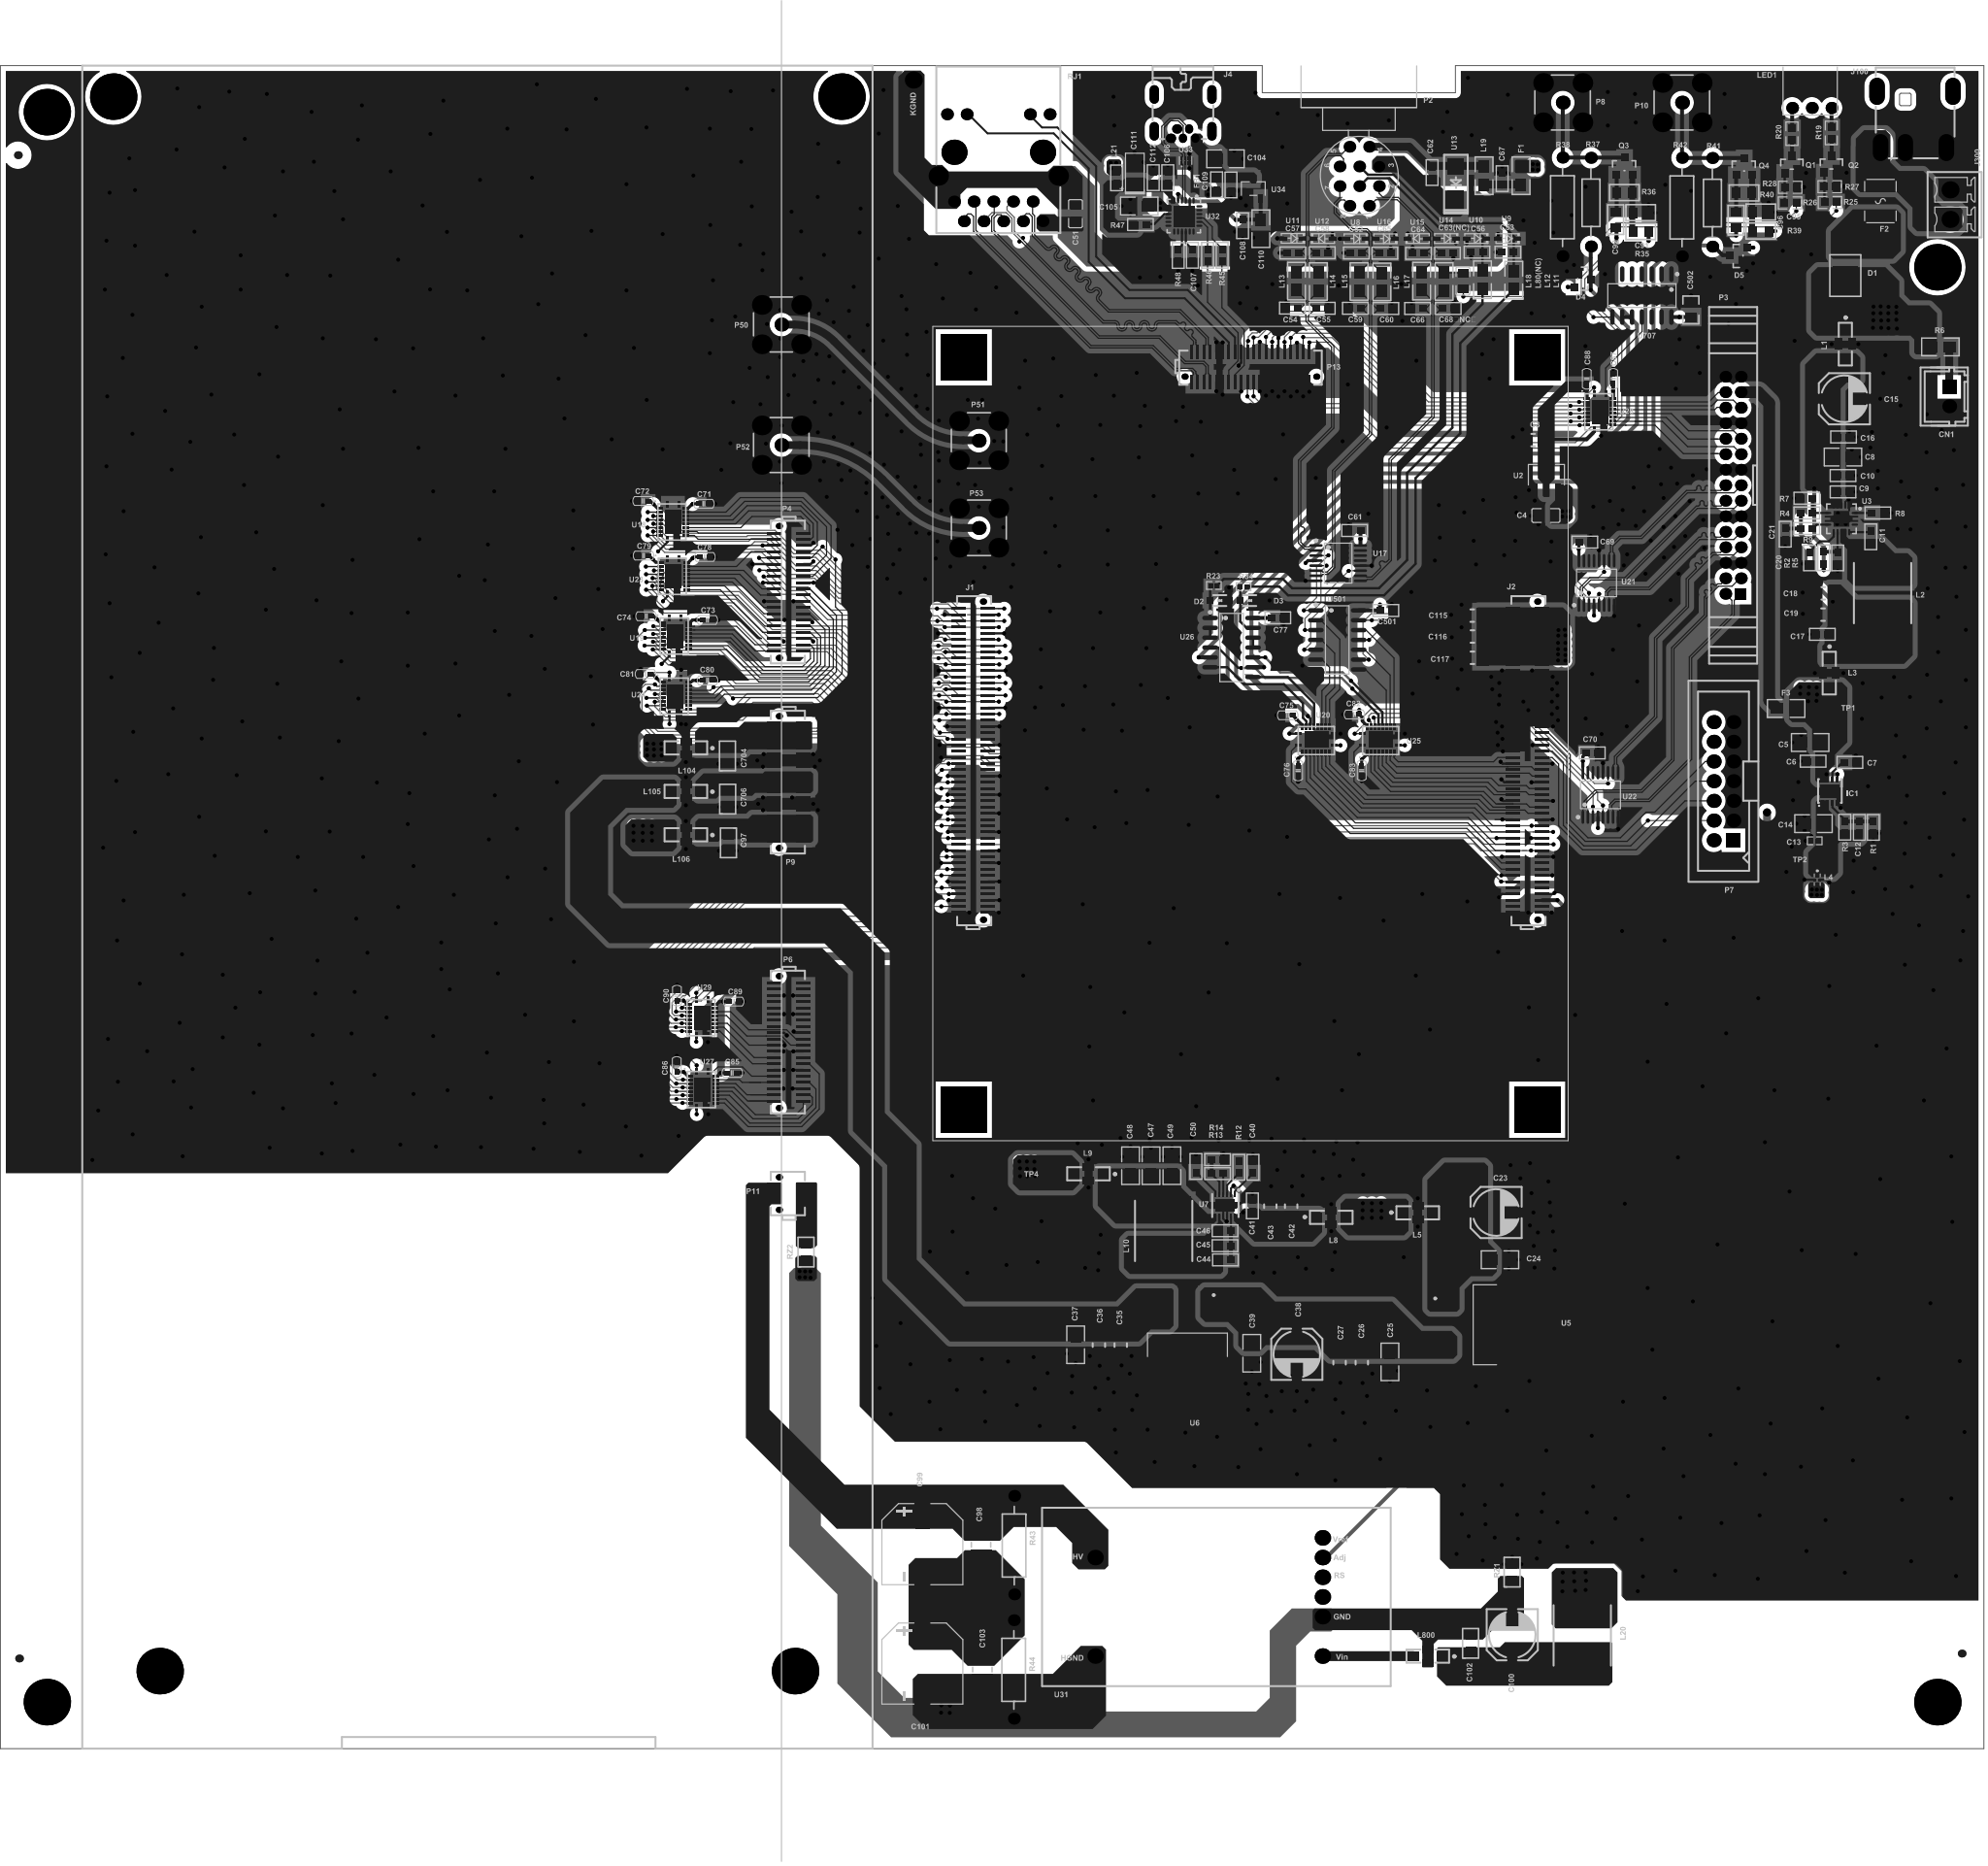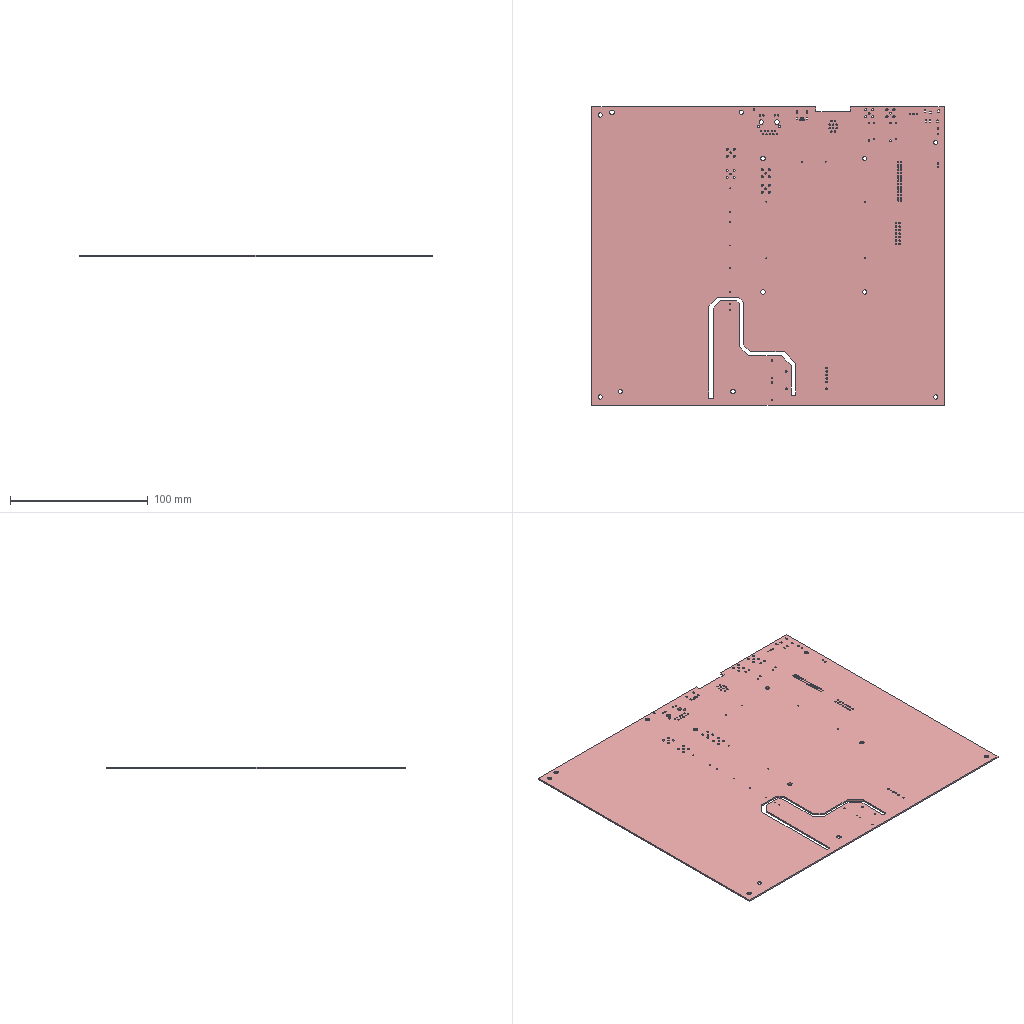Circuit board layout | Altium Designer | box 256 x 217 x 1.1 mm
Layer stack:
# Altium Designer layer stack of  (unit mm; dielectric type: 0 none, 1 core, 2 prepreg, 3 surface material)
index,name,kind,layer,copper_thickness_mm,dielectric_type,dielectric_thickness_mm,dielectric_material,dielectric_constant
0,Top Paste,other,,,,,,
1,Top Overlay,other,,,,,,
2,Top Solder,dielectric,,,3,0.0102,Solder Resist,3.5
3,Top Layer,copper,Top Layer,0.0356,,,,
4,Dielectric1,dielectric,,,1,0.32,FR-4,4.8
5,GND,copper,GND,0.0356,,,,
6,Dielectric5,dielectric,,,2,0.32,FR-4,4.8
7,POWER,copper,POWER,0.0356,,,,
8,Dielectric6,dielectric,,,1,0.32,FR-4,4.8
9,Bottom Layer,copper,Bottom Layer,0.0356,,,,
10,Bottom Solder,dielectric,,,3,0.0102,Solder Resist,3.5
11,Bottom Overlay,other,,,,,,
12,Bottom Paste,other,,,,,,
# drill layer pairs: low layer,high layer
drill_pair,Top Layer,Bottom Layer
Part placement:
Designator,Comment,Layer,Footprint,Center-X(mm),Center-Y(mm),Rotation
U3,#NAME?,TopLayer,VQFN-14_L3.5-W3.5-P0.50-BL-EP_TPS54622RHLT,231.619,152.568,180
R6,0R1%,TopLayer,0805,244.387,174.729,360
CN1,#NAME?,TopLayer,CONN-TH_2P-P2.50_HX25003-2A,245.53,168.328,270
C103,1KV/1nF,TopLayer,3225[1210],120.739,4.193,270
C98,1KV/1nF,TopLayer,3225[1210],120.568,20.289,270
F2,16V 4A,TopLayer,1812,236.646,193.534,270
C3,22uf,TopLayer,1206,191.841,162.818,270
C4,10uf,TopLayer,0805A,193.517,152.937,90
C5,22uF/16V,TopLayer,0805,227.578,123.727,360
C6,100nF,TopLayer,0603,227.959,121.314,90
C7,100nF,TopLayer,0603,232.709,121.162,270
C8,10uF 25V,TopLayer,0805,231.814,160.53,360
C9,4.7uF 25V,TopLayer,0603,231.82,156.036,90
C10,100nF 25V,TopLayer,0603,231.82,158.144,90
C11,100nF 25V,TopLayer,0603,235.402,150.245,360
C12,10nF,TopLayer,0603,233.928,112.78,360
C13,100nF,TopLayer,0402,228.163,111.053,180
C14,22uF/16V,TopLayer,0805,228.01,113.263,360
C15,220UF 25V (D6.3*7.7mm),TopLayer,CAP-SMD-6.3,231.995,168.043,360
C16,100NF 10%,TopLayer,0603,231.89,163.121,90
C17,100nF 25V,TopLayer,0603,229.153,137.672,270
C18,47uF 25V,TopLayer,1206,229.28,143.057,270
C19,47uF 25V,TopLayer,1206,229.255,140.314,270
C20,10nF 25V,TopLayer,0603,227.502,147.527,360
C21,8200pF 25V,TopLayer,0603,224.359,150.582,360
C23,220UF 25V (D6.3*7.7mm),TopLayer,CAP-SMD-6.3,187.042,63.128,360
C24,330nF 10%,TopLayer,0805,187.547,57.038,180
C25,100nF 10%,TopLayer,0805,173.34,43.868,90
C26,47uF 25V,TopLayer,1206,169.814,43.75,180
C27,47uF 25V,TopLayer,1206,166.944,43.75,180
C35,47uF 25V,TopLayer,1206,138.699,46.02,180
C36,47uF 25V,TopLayer,1206,135.88,46.02,180
C37,100nF 10%,TopLayer,0805,132.781,46.071,90
C38,220UF 25V (D6.3*7.7mm),TopLayer,CAP-SMD-6.3,161.325,44.849,270
C39,330nF 10%,TopLayer,0805,155.514,44.979,90
C40,220nF 25V,TopLayer,0603,155.666,68.957,360
C41,2.2uF 25V,TopLayer,0603,155.59,63.978,180
C42,22uF 25V,TopLayer,1206,160.695,63.927,180
C43,22uF 25V,TopLayer,1206,158.003,63.927,180
C44,10uF 16V,TopLayer,0603,152.11,57.019,90
C45,10uF 16V,TopLayer,0603,152.059,58.847,90
C46,10uF 16V,TopLayer,0603,152.059,60.778,90
C47,22uF 16V,TopLayer,0805,142.509,69.16,270
C48,22uF 16V,TopLayer,0805,139.867,69.16,270
C49,22uF 16V,TopLayer,0805,145.201,69.16,270
C50,1uF 25V,TopLayer,0603,148.305,69.067,180
C51,100NF 10%,TopLayer,0805A,132.811,191.952,180
C52,10pF/50V,TopLayer,0603,169.006,186.846,270
C53,10pF/50V,TopLayer,0603,188.564,186.948,270
C54,10pF/50V,TopLayer,0603,160.751,179.734,270
C55,10pF/50V,TopLayer,0603,164.612,179.709,90
C56,10pF/50V,TopLayer,0603,184.576,186.948,270
C57,10pF/50V,TopLayer,0603,160.802,186.846,270
C58,10pF/50V,TopLayer,0603,164.612,186.872,90
C59,10pF/50V,TopLayer,0603,168.879,179.709,270
C60,10pF/50V,TopLayer,0603,172.816,179.684,90
C61,100nF/50V,TopLayer,0603,168.777,151.058,90
C62,10pF/50V,TopLayer,0603,178.785,197.211,180
C63(NC),10pF/50V,TopLayer,0603,180.766,186.821,270
C64,10pF/50V,TopLayer,0603,177.032,186.796,90
C65,10pF/50V,TopLayer,0603,172.689,186.821,270
C66,10pF/50V,TopLayer,0603,176.905,179.684,270
C67,10pF/50V,TopLayer,0603,187.827,196.422,360
C68（NC）,10pF/50V,TopLayer,0603,180.868,179.684,90
C69,100nF/50V,TopLayer,0603,198.495,149.559,270
C70,100nF/50V,TopLayer,0603,199.461,122.381,270
C71,100NF,TopLayer,C0402,84.805,154.512,360
C72,100NF,TopLayer,C0402,76.956,154.868,360
C73,100NF,TopLayer,C0402,85.237,139.526,360
C74,100NF,TopLayer,C0402,77.337,140.009,360
C75,100NF,TopLayer,C0402,160.141,127.233,180
C76,100NF,TopLayer,C0402,161.488,120.121,90
C77,100NF,TopLayer,0603,158.871,139.806,270
C78,100NF,TopLayer,C0402,84.932,147.654,360
C79,100NF,TopLayer,C0402,77.007,147.832,360
C80,100NF,TopLayer,C0402,85.262,131.728,360
C81,100NF,TopLayer,C0402,77.261,132.567,360
C82,100NF,TopLayer,C0402,168.752,127.334,180
C83,100NF,TopLayer,C0402,169.692,120.121,90
C85,100NF,TopLayer,C0402,88.463,81.132,360
C86,100NF,TopLayer,C0402,81.3,81.894,270
C87,100NF,TopLayer,C0402,202.153,170.616,90
C88,100NF,TopLayer,C0402,198.749,170.616,270
C89,100NF,TopLayer,C0402,88.64,90.326,360
C90,100NF,TopLayer,C0402,81.325,91.088,270
C91,100NF 10%,TopLayer,0805R,205.709,192.028,360
C92,150PF 10%,TopLayer,0805R,202.483,191.139,90
C95,100NF 10%,TopLayer,0805R,221.203,192.104,360
C96,150PF 10%,TopLayer,0805R,218.028,191.063,90
C99,500V 10UF,TopLayer,CAP-SMD_BD10.0-L10.3-W10.3-LS11.0-R-RD,112.994,20.366,90
C100,220UF 25V (D6.3*7.7mm),TopLayer,CAP-SMD-6.3,189.129,8.684,90
C101,500V 10UF,TopLayer,CAP-SMD_BD10.0-L10.3-W10.3-LS11.0-R-RD,112.994,4.973,90
C102,100NF 10%,TopLayer,0805R,183.763,7.58,90
C104,10uf,TopLayer,0805,152.115,198.988,180
C105,10uf,TopLayer,0805,140.99,192.892,180
C106,100nF,TopLayer,0603,144.673,196.549,360
C107,4.7uF,TopLayer,0603,147.848,186.542,180
C108,100nF,TopLayer,0603,154.325,190.352,180
C109,2.2uf,TopLayer,0603,152.826,195.609,180
C110,10uf,TopLayer,0805,156.687,189.971,90
C111,4.7UF 10V type A,TopLayer,1005,140.38,197.159,180
C112,0.1uF 10%,TopLayer,0603,142.793,196.549,180
C115,47uF 25V,TopLayer,1206,183.978,140.187,270
C116,47uF 25V,TopLayer,1206,183.978,137.292,90
C117,47uF 25V,TopLayer,1206,183.978,134.548,90
D1,SB1045L,TopLayer,SB1045L,232.118,184.83,270
D2,BV08C,TopLayer,SOD323,151.378,142.041,180
D3,BV08C,TopLayer,SOD323,155.239,142.041,180
D4,BAV99/A7,TopLayer,SOT-23,198.178,183.468,270
D5,BAV99/A7,TopLayer,SOT-23,218.32,186.516,90
F1,Fuse  6V 0.2A,TopLayer,0805,190.266,196.803,90
F3,Fuse  6V 0.2A,TopLayer,0805,224.48,128.112,360
FB1,100R,TopLayer,0603,150.972,195.635,360
IC1,TPL910A,TopLayer,DFN-8_L3.0-W3.0-P0.65-BL-EP2.3,230.128,117.405,360
J1,0.8mm 2*50,TopLayer,板对板座2*50,119.572,121.38,90
J2,0.8mm 2*50,TopLayer,板对板座2*50,191.115,121.38,90
J4,Micro_USB2.0_DIP1,TopLayer,MINI-USB-TH_USB-MINI-2,146.649,204.455,180
L1,YFF31HC2A105MT000N,TopLayer,FILTER-SMD_4P-L3.2-W1.6-L_YFF31HC,232.118,175.089,270
L2,SLF0705-2R2MTT (2.2uH 6A),TopLayer,IND-SMD_L7.8-W7.0-A,236.926,142.988,90
L3,YFF31HC2A105MT000N,TopLayer,FILTER-SMD_4P-L3.2-W1.6-L_YFF31HC,230.042,132.672,270
L4,YFF15PC0G435MT000N,TopLayer,FILTER-SMD_4P-L1.0-W0.5-L,228.493,106.033,270
L5,YFF31HC2A105MT000N,TopLayer,FILTER-SMD_4P-L3.2-W1.6-L_YFF31HC,176.931,63.087,360
L8,YFF31HC2A105MT000N,TopLayer,FILTER-SMD_4P-L3.2-W1.6-L_YFF31HC,165.771,62.505,360
L9,YFF31HC2A105MT000N,TopLayer,FILTER-SMD_4P-L3.2-W1.6-L_YFF31HC,134.436,68.118,180
L10,XRCD54-4R7M(4.7uH 2A SMD,4.5x5.2mm),TopLayer,IND-SMD_L7.8-W7.0-A,144.139,60.753,270
L11,600Ω-1.3A,TopLayer,0805,189.326,183.341,90
L12,600Ω-1.3A,TopLayer,0805,185.287,183.392,90
L13,600Ω-1.3A,TopLayer,0805,161.284,183.214,90
L14,600Ω-1.3A,TopLayer,0805,164.104,183.163,90
L15,600Ω-1.3A,TopLayer,0805,169.362,183.163,90
L16,600Ω-1.3A,TopLayer,0805,172.308,183.113,90
L17,600Ω-1.3A,TopLayer,0805,177.439,183.214,90
L18,600Ω-1.3A,TopLayer,0805,180.334,183.163,90
L19,600Ω-1.3A,TopLayer,0805,185.491,196.803,90
L20,XRCD54-4R7M(4.7uH 2A SMD,4.5x5.2mm),TopLayer,IND-SMD_L7.8-W7.0-A,198.165,8.597,270
L21,600Ω-1.3A,TopLayer,0603,138.069,196.524,180
LED1,LED white body, red/green bicolour(F3/common anode) with 3mm single-hole square LED right-angle holder(7*6.4*7.4mm),TopLayer,DIP3B,227.796,205.546,90
P2,Header 10,TopLayer,2B-10,169.387,196.727,360
P4,Header 20X2,TopLayer,N0.8mm/40Pin-Plug,95.733,143.13,270
P6,Header 20X2,TopLayer,N0.8mm/40Pin-Plug,95.733,85.104,270
P7,Header 7X2,TopLayer,IDC-TH_14P-P2.54-V-R2-C7-S2.54,216.402,118.739,90
P8,RF connector SMB-JWHD SMB right-angle male,TopLayer,DIP-P,195.651,206.227,90
P9,Header 20X2,TopLayer,N0.8mm/40Pin-Plug,95.733,118.616,270
P10,RF connector SMB-JWHD SMB right-angle male,TopLayer,DIP-P,211.043,206.227,90
P11,Header 4X2,TopLayer,N0.8mm/8Pin-SOCKET,95.733,65.573,270
P13,Header 20X2,TopLayer,N0.8mm/40Pin-Plug,155.343,172.152,360
P50,Analog output,TopLayer,DIP-P,94.813,177.607,90
P51,AD input,TopLayer,DIP-P,120.263,162.64,360
P52,gain,TopLayer,DIP-P,94.813,162.067,90
P53,,TopLayer,DIP-P,120.273,151.38,360
Q1,MMBT3904LT1(1AM),TopLayer,SOT23,225.243,198.244,360
Q2,MMBT3904LT1(1AM),TopLayer,SOT23,230.348,198.269,360
Q3,MMBT3906/2A,TopLayer,SOT-23,203.626,198.06,360
Q4,MMBT3906/2A,TopLayer,SOT-23,219.069,198.01,360
R1,10K 1%,TopLayer,0603,235.732,112.78,180
R2,35.7K 1%,TopLayer,0603,229.331,147.553,180
R3,31.3K 1%,TopLayer,0603,232.049,112.805,360
R4,56K 1%,TopLayer,0603,227.147,153.318,270
R5,8.06K 1%,TopLayer,0603,231.134,147.527,360
R7,10K 1%,TopLayer,0603,227.147,155.223,270
R8,80.6K 1%,TopLayer,0603,236.316,153.318,90
R9,1.69K 1%,TopLayer,0603,227.147,151.312,270
R12,100K 1%,TopLayer,0603,153.837,68.957,360
R13,143K 1%,TopLayer,0603,151.094,68.144,90
R14,24K 1%,TopLayer,0603,151.094,69.947,90
R19,100R 5%,TopLayer,0603A,230.336,202.269,180
R20,100R 5%,TopLayer,0603A,225.256,202.168,180
R23,1K,TopLayer,0402,150.616,143.971,360
R25,2K 5%,TopLayer,0603A,230.185,193.372,270
R26,2K 5%,TopLayer,0603A,225.029,193.322,270
R27,2K 5%,TopLayer,0603A,230.158,195.411,270
R28,2K 5%,TopLayer,0603A,225.052,195.335,270
R34,1K,TopLayer,0402,154.452,143.819,180
R35,100R 5%,TopLayer,0805R,205.709,189.59,360
R36,100R 5%,TopLayer,0805R,203.601,194.644,180
R37,100R 1% 1/4W,TopLayer,AXIAL-0.45,199.283,193.4,90
R38,49.9R 1% 1/4W,TopLayer,AXIAL-0.5,195.625,192.79,90
R39,100R 5%,TopLayer,0805R,221.203,189.666,360
R40,100R 5%,TopLayer,0805R,219.044,194.593,180
R41,100R 1% 1/4W,TopLayer,AXIAL-0.45,214.955,193.374,90
R42,49.9R 1% 1/4W,TopLayer,AXIAL-0.5,211.043,192.765,90
R43,2.2M 5% 1/4W,TopLayer,AXIAL-0.5,124.856,20.239,90
R44,2.2M 5% 1/4W,TopLayer,AXIAL-0.5,124.805,4.212,90
R45,100R,TopLayer,0603,151.683,186.542,360
R46,100R,TopLayer,0603,149.804,186.542,360
R47,10K,TopLayer,0603,141.142,190.504,270
R48,10K,TopLayer,0603,146.019,186.516,360
RJ1,HY911130A,TopLayer,HY911130A,122.799,197.831,0
TP1,,TopLayer,TP1,230.017,128.122,270
TP2,,TopLayer,TP1,228.493,108.716,270
TP4,,TopLayer,TP1,129.382,68.133,180
U2,AMS1117S-1.8,TopLayer,SOT-89-3_L4.5-W2.5-P1.50-LS4.2-BR,193.536,156.25,270
U5,L7809CD2T-TR(ST),TopLayer,TO-263-2_L10.0-W9.1-P5.08-LS15.2-TL,185.568,48.656,360
U6,L7806CD2T-TR(ST),TopLayer,TO-263-2_L10.0-W9.1-P5.08-LS15.2-TL,147.208,46.094,270
U7,#NAME?,TopLayer,TDFN-12_L3.0-W3.0-P0.50-BL-EP,152.079,64.026,180
U8,BV05C,TopLayer,SOD-323,168.93,188.675,360
U9,BV05C,TopLayer,SOD-323,188.539,188.701,360
U10,BV05C,TopLayer,SOD-323,184.5,188.701,360
U11,BV05C,TopLayer,SOD-323,160.827,188.726,360
U12,BV05C,TopLayer,SOD-323,164.688,188.701,180
U13,SMBJ33CA /33V,TopLayer,DO-214AC(SMA),181.858,195.941,90
U14,BV05C,TopLayer,SOD-323,180.614,188.701,360
U15,BV05C,TopLayer,SOD-323,176.905,188.701,180
U16,BV05C,TopLayer,SOD-323,172.765,188.675,360
U17,#NAME?,TopLayer,TSSOP-16_L5.0-W4.4-P0.65-LS6.4-BL,166.665,146.852,270
U18,TXB0108RGYR,TopLayer,QFN20,80.803,152.177,270
U19,TXB0108RGYR,TopLayer,QFN20,81.11,137.471,270
U20,TXB0108RGYR,TopLayer,QFN20,163.814,124.111,360
U21,#NAME?,TopLayer,TSSOP-16_L5.0-W4.4-P0.65-LS6.4-BL,200.008,144.297,360
U22,#NAME?,TopLayer,TSSOP-16_L5.0-W4.4-P0.65-LS6.4-BL,200.517,116.967,360
U23,TXB0108RGYR,TopLayer,QFN20,80.856,145.167,270
U24,TXB0108RGYR,TopLayer,QFN20,81.11,129.724,270
U25,TXB0108RGYR,TopLayer,QFN20,172.119,124.111,360
U26,74HC14D,TopLayer,SO-14,152.903,135.97,270
U27,TXB0108RGYR,TopLayer,QFN20,84.615,79,270
U28,TXB0108RGYR,TopLayer,QFN20,200.439,166.385,270
U29,TXB0108RGYR,TopLayer,QFN20,84.564,88.271,270
U31,DW-N601-5CN2,TopLayer,DW-N601-5CN2,149.962,13.559,180
U32,CP2104,TopLayer,QFN-24_L4.0-W4.0-P0.50-BL-EP2.7,146.751,191.603,180
U33,RCLAMP0522P,TopLayer,DFN-1610-6_L1.6-W1.0-P0.50-BL,146.976,198.754,360
U34,XC6206P182MR,TopLayer,SOT-23-3_L2.9-W1.6-P1.90-LS2.8-BR,155.707,195.143,270
C501,100nF/50V,TopLayer,0603,172.816,140.745,270
U501,74HC14D,TopLayer,SO-14,166.54,136.95,270
C97,10uF  25V 10%,TopLayer,0805R,87.955,110.789,270
C502,100nF/50V,TopLayer,0603,212.211,179.496,360
C704,10uF  25V 10%,TopLayer,0805R,87.853,121.991,90
C706,10uF  25V 10%,TopLayer,0805R,87.878,116.428,90
J100,DC-044A-A250,TopLayer,DC-IN-TH_DC-044A-A250,241.112,204.059,270
L80(NC),600Ω-1.3A,TopLayer,0805,182.814,183.263,180
L104,YFF31HC2A105MT000N,TopLayer,FILTER-SMD_4P-L3.2-W1.6-L_YFF31HC,82.472,123.032,180
L105,YFF31HC2A105MT000N,TopLayer,FILTER-SMD_4P-L3.2-W1.6-L_YFF31HC,82.472,117.419,180
L106,YFF31HC2A105MT000N,TopLayer,FILTER-SMD_4P-L3.2-W1.6-L_YFF31HC,82.472,111.831,180
L800,YFF31HC2A105MT000N,TopLayer,FILTER-SMD_4P-L3.2-W1.6-L_YFF31HC,178.23,5.929,180
P3,MTE220-30SL,TopLayer,CONN-TH_MTE220-30SL,217.638,156.895,90
RZ1,0R,TopLayer,0805R,189.123,16.758,90
RZ2,0R,TopLayer,0805R,97.988,58.024,90
U707,74HC14D,TopLayer,SO-14,205.861,181.35,180
J300,WJ15EDGVC-3.81-2P,TopLayer,CONN-TH_WJ15EDGVC-3.81-2P,245.638,193.076,90
Pad and via stacks, first 69 of 85 lines:
# Altium Designer via and pad stacks of  (unit mm). Each distinct definition once, with the count of objects using it.
# via: kind,start_layer,end_layer,hole_mm,diameter_mm,mode(0 simple;1 top-mid-bottom;2 full stack),diameter_per_layer,count,example_net
# pad: kind,layer,hole_mm,hole_type(0 round;1 square;2 slot),plating,top_size,top_shape(1 round;2 rect;3 octagon;9 rounded rect),mid_size,bottom_size,mode,footprint,size_per_layer,count,example
pad,Multi-Layer,1.1,0,plated,1.8x1.8,1,1.8x1.8,1.8x1.8,0,CONN-TH_2P-P2.50_HX25003-2A,,1,CN1.2
pad,Multi-Layer,1.1,0,plated,1.8x1.8,2,1.8x1.8,1.8x1.8,0,CONN-TH_2P-P2.50_HX25003-2A,,1,CN1.1
pad,Multi-Layer,3.2,0,plated,6x6,2,6x6,6x6,0,,,4,0
pad,Multi-Layer,1.016,0,plated,1.524x1.524,1,1.524x1.524,1.524x1.524,0,AXIAL-0.5,,8,R44.1
pad,Multi-Layer,1.2,0,plated,2x2,1,2x2,2x2,0,DW-N601-5CN2,,8,U31.6
pad,Multi-Layer,0.68,0,plated,0.8x0.8,1,0.8x0.8,0.8x0.8,0,N0.8mm/8Pin-SOCKET,,2,P11.0
pad,Multi-Layer,0.9144,0,plated,1.524x1.524,1,1.524x1.524,1.524x1.524,0,HY911130A,,14,RJ1.10
pad,Multi-Layer,1.8,0,plated,2.5x2.5,1,2.5x2.5,2.5x2.5,0,HY911130A,,2,RJ1.16
pad,Multi-Layer,3.25,0,unplated,3.25x3.25,1,3.25x3.25,3.25x3.25,0,HY911130A,,2,RJ1.
pad,Multi-Layer,1.1,0,plated,1.8x1.8,2,1.8x1.8,1.8x1.8,0,IDC-TH_14P-P2.54-V-R2-C7-S2.54,,1,P7.1
pad,Multi-Layer,1.1,0,plated,1.8x1.8,1,1.8x1.8,1.8x1.8,0,IDC-TH_14P-P2.54-V-R2-C7-S2.54,,13,P7.2
pad,Multi-Layer,0.68,0,plated,0.8x0.8,1,0.8x0.8,0.8x0.8,0,N0.8mm/40Pin-Plug,,8,P13.0
pad,Multi-Layer,0.68,0,plated,0.8x0.8,1,0.8x0.8,0.8x0.8,0,\u00B0\u00E5\u00B6\u00D4\u00B0\u00E5\u00D7\u00F92*50,,4,J1.0
pad,Multi-Layer,1.016,0,plated,1.524x1.524,1,1.524x1.524,1.524x1.524,0,AXIAL-0.45,,4,R37.2
pad,Multi-Layer,1.524,0,plated,2.54x2.54,1,2.54x2.54,2.54x2.54,0,DIP-P,,24,P8.1
pad,Multi-Layer,1.143,0,plated,1.778x1.778,1,1.778x1.778,1.778x1.778,0,DIP-P,,6,P8.5
pad,Multi-Layer,1.016,0,plated,1.524x1.524,1,1.397x1.397,1.524x1.524,1,DIP3B,,3,LED1.3
pad,Multi-Layer,1.016,0,plated,1.397x1.397,1,1.524x1.524,1.524x1.524,1,2B-10,,10,P2.6
pad,Multi-Layer,0.8,2,plated,2.4x1.2,1,2.4x1.2,2.4x1.2,0,MINI-USB-TH_USB-MINI-2,,4,J4.0
pad,Multi-Layer,0.8,0,plated,1.2x1.041,1,1.2x1.041,1.2x1.041,0,MINI-USB-TH_USB-MINI-2,,3,J4.1
pad,Multi-Layer,0.8,0,plated,1.2x1.2,1,1.2x1.2,1.2x1.2,0,MINI-USB-TH_USB-MINI-2,,2,J4.4
pad,Multi-Layer,3.2,0,plated,6x6,1,6x6,6x6,0,,,8,0
pad,Multi-Layer,1.2,0,plated,2.2x2.2,1,2.2x2.2,2.2x2.2,0,,,1,1
pad,Multi-Layer,0.9,0,plated,1.5x1.5,1,1.5x1.5,1.5x1.5,0,CONN-TH_MTE220-30SL,,29,P3.30
pad,Multi-Layer,0.9,0,plated,1.5x1.5,2,1.5x1.5,1.5x1.5,0,CONN-TH_MTE220-30SL,,1,P3.1
pad,Multi-Layer,0.9,2,plated,3.5x2,1,3.5x2,3.5x2,0,DC-IN-TH_DC-044A-A250,,5,J100.1
pad,Multi-Layer,1.25,0,plated,2.2x2.2,1,2.2x2.2,2.2x2.2,0,CONN-TH_WJ15EDGVC-3.81-2P,,2,J300.2
pad,Top Layer,0,0,plated,0.85x0.28,1,0.85x0.28,0.85x0.28,0,VQFN-14_L3.5-W3.5-P0.50-BL-EP_TPS54622RHLT,,14,U3.9
pad,Top Layer,0,0,plated,2.592x1.219,1,2.592x1.219,2.592x1.219,0,VQFN-14_L3.5-W3.5-P0.50-BL-EP_TPS54622RHLT,,1,U3.15
pad,Top Layer,0,0,plated,1.524x1.27,2,1.524x1.27,1.524x1.27,0,0805,,50,R6.1
pad,Top Layer,0,0,plated,1.27x1.016,2,1.27x1.016,1.27x1.016,0,0805R,,28,C102.1
pad,Top Layer,0,0,plated,4.8x1.8,2,4.8x1.8,4.8x1.8,0,CAP-SMD_BD10.0-L10.3-W10.3-LS11.0-R-RD,,4,C101.1
pad,Top Layer,0,0,plated,3x1,2,3x1,3x1,0,CAP-SMD-6.3,,8,C100.1
pad,Top Layer,0,0,plated,3.5x7,2,3.5x7,3.5x7,0,IND-SMD_L7.8-W7.0-A,,6,L20.2
pad,Top Layer,0,0,plated,0.3x1.8,2,0.3x1.8,0.3x1.8,0,N0.8mm/8Pin-SOCKET,,8,P11.7
pad,Top Layer,0,0,plated,1.27x1.016,2,1.27x1.016,1.27x1.016,0,0805A,,4,C51.1
pad,Top Layer,0,0,plated,0.8x0.8,2,0.8x0.8,0.8x0.8,0,SOD323,,4,D3.1
pad,Top Layer,0,0,plated,0.5657x0.54,2,0.5657x0.54,0.5657x0.54,0,0402,,6,R34.1
pad,Top Layer,0,0,plated,1.829x1.575,2,1.829x1.575,1.829x1.575,0,1206,,24,C115.1
pad,Top Layer,0,0,plated,0.574x2.038,1,0.574x2.038,0.574x2.038,0,SO-14,,42,U26.1
pad,Top Layer,0,0,plated,0.3x1.8,2,0.3x1.8,0.3x1.8,0,N0.8mm/40Pin-Plug,,160,P13.40
pad,Top Layer,0,0,plated,0.3x1.8,2,0.3x1.8,0.3x1.8,0,\u00B0\u00E5\u00B6\u00D4\u00B0\u00E5\u00D7\u00F92*50,,200,J1.B41
pad,Top Layer,0,0,plated,0.889x0.889,2,0.889x0.889,0.889x0.889,0,SOT-23,,12,D4.2
pad,Top Layer,0,0,plated,0.635x0.508,2,0.635x0.508,0.635x0.508,0,C0402,,36,C87.1
pad,Top Layer,0,0,plated,0.3048x0.8128,2,0.3048x0.8128,0.3048x0.8128,0,QFN20,,180,U28.12
pad,Top Layer,0,0,plated,3.048x2.032,2,3.048x2.032,3.048x2.032,0,QFN20,,9,U28.11
pad,Top Layer,0,0,plated,0.343x1.732,1,0.343x1.732,0.343x1.732,0,TSSOP-16_L5.0-W4.4-P0.65-LS6.4-BL,,48,U22.1
pad,Top Layer,0,0,plated,0.9652x0.9652,2,0.9652x0.9652,0.9652x0.9652,0,0603A,,12,R27.1
pad,Top Layer,0,0,plated,1.016x0.889,2,1.016x0.889,1.016x0.889,0,SOT23,,6,Q2.2
pad,Top Layer,0,0,plated,0.9x0.5,2,0.9x0.5,0.9x0.5,0,SOD-323,,16,U14.1
pad,Top Layer,0,0,plated,2.032x2.032,2,2.032x2.032,2.032x2.032,0,DO-214AC(SMA),,2,U13.2
pad,Top Layer,0,0,plated,1.829x1.575,2,1.829x1.575,1.829x1.575,0,1005,,2,C111.1
pad,Top Layer,0,0,plated,1.07x0.6,2,1.07x0.6,1.07x0.6,0,SOT-23-3_L2.9-W1.6-P1.90-LS2.8-BR,,3,U34.1
pad,Top Layer,0,0,plated,0.2x0.4,2,0.2x0.4,0.2x0.4,0,DFN-1610-6_L1.6-W1.0-P0.50-BL,,4,U33.6
pad,Top Layer,0,0,plated,0.38x0.42,2,0.38x0.42,0.38x0.42,0,DFN-1610-6_L1.6-W1.0-P0.50-BL,,2,U33.4
pad,Top Layer,0,0,plated,2.7x2.7,2,2.7x2.7,2.7x2.7,0,QFN-24_L4.0-W4.0-P0.50-BL-EP2.7,,1,U32.25
pad,Top Layer,0,0,plated,0.8x0.28,1,0.8x0.28,0.8x0.28,0,QFN-24_L4.0-W4.0-P0.50-BL-EP2.7,,12,U32.24
pad,Top Layer,0,0,plated,0.28x0.8,1,0.28x0.8,0.28x0.8,0,QFN-24_L4.0-W4.0-P0.50-BL-EP2.7,,12,U32.18
pad,Top Layer,0,0,plated,2.159x2.159,1,2.159x2.159,2.159x2.159,0,TP1,,3,TP4.1
pad,Top Layer,0,0,plated,1.6x2.5,2,1.6x2.5,1.6x2.5,0,TDFN-12_L3.0-W3.0-P0.50-BL-EP,,1,U7.13
pad,Top Layer,0,0,plated,0.25x0.6,2,0.25x0.6,0.25x0.6,0,TDFN-12_L3.0-W3.0-P0.50-BL-EP,,12,U7.12
pad,Top Layer,0,0,plated,1.4x0.9,2,1.4x0.9,1.4x0.9,0,FILTER-SMD_4P-L3.2-W1.6-L_YFF31HC,,18,L9.4
pad,Top Layer,0,0,plated,1.3x1.2,2,1.3x1.2,1.3x1.2,0,FILTER-SMD_4P-L3.2-W1.6-L_YFF31HC,,18,L9.3
pad,Top Layer,0,0,plated,7.181x10.566,2,7.181x10.566,7.181x10.566,0,TO-263-2_L10.0-W9.1-P5.08-LS15.2-TL,,2,U6.4
pad,Top Layer,0,0,plated,3.358x1.134,2,3.358x1.134,3.358x1.134,0,TO-263-2_L10.0-W9.1-P5.08-LS15.2-TL,,4,U6.3
pad,Top Layer,0,0,plated,0.3x0.3,2,0.3x0.3,0.3x0.3,0,FILTER-SMD_4P-L1.0-W0.5-L,,2,L4.4
Copper pours:
name,layer,net,type(0 solid;1 hatched;2 none)
Bottom Layer-No Net,Top Layer,13V,0
Bottom Layer-No Net,Top Layer,13V,0
Bottom Layer-No Net,Top Layer,A6V,0
Bottom Layer-No Net,Top Layer,-5.4V,0
Bottom Layer-No Net,Top Layer,-5.4V,0
Bottom Layer-No Net,Top Layer,NetF2_1,0
Bottom Layer-No Net,Top Layer,NetD1_1,0
Bottom Layer-No Net,Top Layer,9V 1.5A,0
Bottom Layer-No Net,Top Layer,13V,0
Bottom Layer-No Net,Top Layer,NetC97_1,0
Bottom Layer-No Net,Top Layer,A6V4,0
Bottom Layer-No Net,Top Layer,NetC704_2,0
Bottom Layer-No Net,Top Layer,D5V,0
Bottom Layer-No Net,Top Layer,13V,0
Bottom Layer-No Net,Top Layer,3V3,0
Bottom Layer-No Net,Top Layer,3V3,0
Bottom Layer-No Net,Top Layer,3V3,0
Bottom Layer-No Net,Top Layer,13V,0
Bottom Layer-No Net,Top Layer,NetC12_2,0
Bottom Layer-No Net,Top Layer,NetC8_1,0
Bottom Layer-No Net,Top Layer,NetC17_1,0
Bottom Layer-No Net,Top Layer,NetC11_2,0
Bottom Layer-No Net,Top Layer,NetC98_2,0
Bottom Layer-No Net,Top Layer,NetC23_1,0
Bottom Layer-No Net,Top Layer,NetC41_1,0
Bottom Layer-No Net,Top Layer,NetC44_1,0
Bottom Layer-No Net,Top Layer,NetC47_2,0
Bottom Layer-No Net,Top Layer,KGND,0
Bottom Layer-No Net,Top Layer,NetC105_1,0
Bottom Layer-No Net,Top Layer,NetC105_1,0
Bottom Layer-No Net,Top Layer,C3.3V,0
Bottom Layer-No Net,Top Layer,USB_5VIN,0
Bottom Layer-No Net,Top Layer,NetC51_1,0
Bottom Layer-No Net,Top Layer,VCC1V8,0
Bottom Layer-No Net,Top Layer,D5V,0
Bottom Layer-No Net,Top Layer,HT,0
Bottom Layer-No Net,Top Layer,KGND,0
Bottom Layer-No Net,Top Layer,NetC100_1,0
Bottom Layer-No Net,Top Layer,NetP11_2,0
Bottom Layer-No Net,Top Layer,HGND,0
Bottom Layer-No Net,Top Layer,HGND,0
Bottom Layer-No Net,Top Layer,HGND,0
Bottom Layer-No Net,Top Layer,DGND,0
Bottom Layer-No Net,Bottom Layer,KGND,0
Bottom Layer-No Net,Bottom Layer,NetC105_1,0
Bottom Layer-No Net,Bottom Layer,HGND,0
Bottom Layer-No Net,Bottom Layer,DGND,0
Design rules, without the lines most boards share:
# Altium Designer design rules of  (exported by Altium Designer, unit mm)
# columns: name | kind | enabled | priority | scope1 | scope2 | descriptor | typed fields (field=value)
Clearance_1 | 0 | enabled | 2 | INPOLYGON | All | Clearance Constraint (Gap=6mil) (INPOLYGON),(All) | gap=0.1524
Clearance | 0 | enabled | 3 | All | All | Clearance Constraint (Gap=6mil) (All),(All) | gap=0.1524
PlaneConnect | 6 | enabled | 1 | All | All | Power Plane Connect Rule(Direct Connect )(Expansion=20mil) (Conductor Width=10mil) (Air Gap=10mil) (Entries=4) (All) | relief_conductor_width=0.254 relief_entries=4 relief_expansion=0.508
PlaneClearance | 12 | enabled | 1 | All | All | Power Plane Clearance (Clearance =6mil) (All) | clearance=0.1524
PolygonConnect | 20 | enabled | 1 | All | All | Polygon Connect Rule(Direct Connect )(Conductor Width=10mil) (Relief Angle=90 Angle) (Entries=4) (Air Gap Width=10mil) (All),(All) | connect_style(0=relief,1=direct,2=none)=1 relief_conductor_width=0.254 relief_entries=4
Width | 2 | enabled | 1 | All | All | Width Constraint (Min=6mil) (Max=100mil) (Preferred=6mil) (All) |
RoutingVias | 11 | enabled | 1 | All | All | Routing Via (MinHoleWidth=12mil) (MaxHoleWidth=12mil) (PreferredHoleWidth=12mil) (MinWidth=20mil) (MaxWidth=20mil) (PreferedWidth=20mil) (All) | via_min_hole=0.3048 via_max_hole=0.3048 via_preferred_diameter=0.508 via_preferred_hole=0.3048
SolderMaskExpansion | 13 | enabled | 1 | All | All | Solder Mask Expansion (Expansion =4mil) (All) | expansion=0.1016
HoleSize | 42 | enabled | 1 | All | All | Hole Size Constraint (Min=1mil) (Max=500mil) (All) |
DiffPairsRouting | 51 | enabled | 1 | All | All | Differential Pairs Uncoupled Length using the Gap Constraints (Min=6mil) (Max=6mil) (Prefered=6mil)  and Width Constraints (Min=15mil) (Max=15mil) (Prefered=15mil) (All) |
HoleToHoleClearance | 52 | enabled | 1 | All | All | Hole To Hole Clearance (Gap=0mil) (All),(All) | gap=0
MinimumSolderMaskSliver | 53 | enabled | 1 | All | All | Minimum Solder Mask Sliver (Gap=0mil) (All),(All) |
SilkscreenOverComponentPads | 54 | enabled | 1 | IsPad | All | Silk To Solder Mask (Clearance=0mil) (IsPad),(All) |
SilkToSilkClearance | 55 | enabled | 1 | All | All | Silk to Silk (Clearance=0mil) (All),(All) |
Clearance_2 | 0 | enabled | 1 | HASPAD('FREE-MARK') | All | Clearance Constraint (Gap=50mil) (HASPAD('FREE-MARK')),(All) | gap=1.27